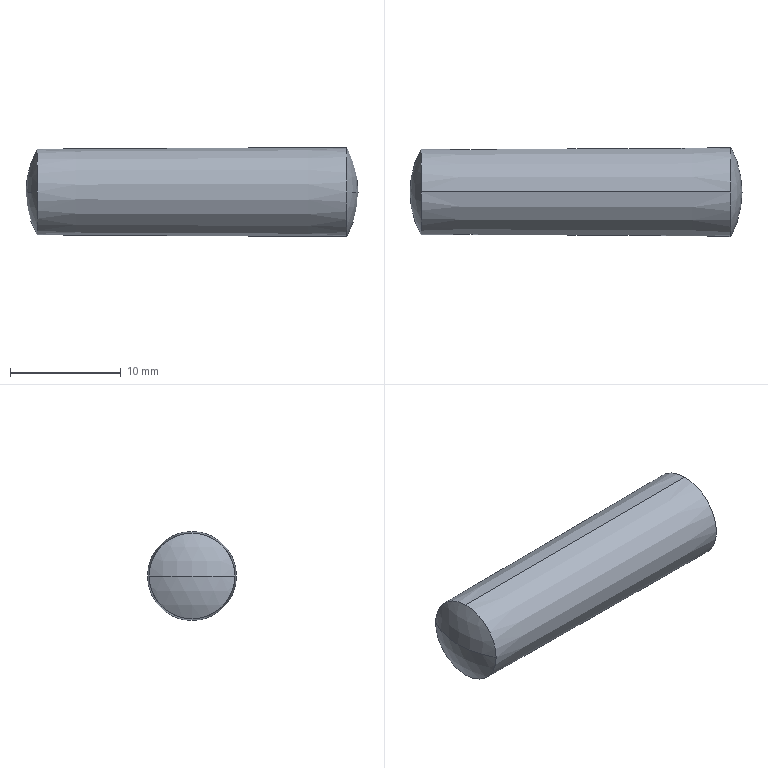Part | SolidWorks | features Revolution 1 | 1 solid | 6 faces | box 30 x 8.048 x 8.048 mm | volume 1422 mm3 | sphere 4 | cone 2
STEP:
#1=CARTESIAN_POINT('',(-7.,0.,3.873));
#2=VERTEX_POINT('',#1);
#3=CARTESIAN_POINT('',(-7.,3.873,0.));
#4=VERTEX_POINT('',#3);
#5=CARTESIAN_POINT('',(-7.,0.,0.));
#6=DIRECTION('',(-1.,0.,0.));
#7=DIRECTION('',(0.,0.,1.));
#8=AXIS2_PLACEMENT_3D('',#5,#6,#7);
#9=CIRCLE('',#8,3.873);
#10=EDGE_CURVE('',#2,#4,#9,.T.);
#11=ORIENTED_EDGE('',*,*,#10,.F.);
#12=CARTESIAN_POINT('',(21.,0.,4.024));
#13=VERTEX_POINT('',#12);
#14=CARTESIAN_POINT('',(21.,0.,4.024));
#15=DIRECTION('',(1.,0.,0.005398));
#16=VECTOR('',#15,1000.);
#17=LINE('',#14,#16);
#18=EDGE_CURVE('',#2,#13,#17,.T.);
#19=ORIENTED_EDGE('',*,*,#18,.T.);
#20=CARTESIAN_POINT('',(21.,4.024,0.));
#21=VERTEX_POINT('',#20);
#22=CARTESIAN_POINT('',(21.,0.,0.));
#23=DIRECTION('',(-1.,0.,0.));
#24=DIRECTION('',(0.,0.,1.));
#25=AXIS2_PLACEMENT_3D('',#22,#23,#24);
#26=CIRCLE('',#25,4.024);
#27=EDGE_CURVE('',#13,#21,#26,.T.);
#28=ORIENTED_EDGE('',*,*,#27,.T.);
#29=CARTESIAN_POINT('',(21.,0.,-4.024));
#30=VERTEX_POINT('',#29);
#31=CARTESIAN_POINT('',(21.,0.,0.));
#32=DIRECTION('',(-1.,0.,0.));
#33=DIRECTION('',(0.,0.,1.));
#34=AXIS2_PLACEMENT_3D('',#31,#32,#33);
#35=CIRCLE('',#34,4.024);
#36=EDGE_CURVE('',#21,#30,#35,.T.);
#37=ORIENTED_EDGE('',*,*,#36,.T.);
#38=CARTESIAN_POINT('',(-7.,0.,-3.873));
#39=VERTEX_POINT('',#38);
#40=CARTESIAN_POINT('',(21.,0.,-4.024));
#41=DIRECTION('',(1.,0.,-0.005398));
#42=VECTOR('',#41,1000.);
#43=LINE('',#40,#42);
#44=EDGE_CURVE('',#39,#30,#43,.T.);
#45=ORIENTED_EDGE('',*,*,#44,.F.);
#46=CARTESIAN_POINT('',(-7.,0.,0.));
#47=DIRECTION('',(-1.,0.,0.));
#48=DIRECTION('',(0.,0.,1.));
#49=AXIS2_PLACEMENT_3D('',#46,#47,#48);
#50=CIRCLE('',#49,3.873);
#51=EDGE_CURVE('',#4,#39,#50,.T.);
#52=ORIENTED_EDGE('',*,*,#51,.F.);
#53=EDGE_LOOP('',(#11,#19,#28,#37,#45,#52));
#54=FACE_OUTER_BOUND('',#53,.T.);
#55=CARTESIAN_POINT('',(21.,0.,0.));
#56=DIRECTION('',(1.,0.,0.));
#57=DIRECTION('',(0.,0.,-1.));
#58=AXIS2_PLACEMENT_3D('',#55,#56,#57);
#59=CONICAL_SURFACE('',#58,4.024,0.005398);
#60=ADVANCED_FACE('',(#54),#59,.T.);
#61=CARTESIAN_POINT('',(22.,0.,0.));
#62=VERTEX_POINT('',#61);
#63=CARTESIAN_POINT('',(13.403,0.,0.));
#64=DIRECTION('',(0.,0.,1.));
#65=DIRECTION('',(1.,0.,0.));
#66=AXIS2_PLACEMENT_3D('',#63,#64,#65);
#67=CIRCLE('',#66,8.597);
#68=EDGE_CURVE('',#62,#21,#67,.T.);
#69=ORIENTED_EDGE('',*,*,#68,.F.);
#70=CARTESIAN_POINT('',(21.,-4.024,0.));
#71=VERTEX_POINT('',#70);
#72=CARTESIAN_POINT('',(13.403,0.,0.));
#73=DIRECTION('',(0.,0.,-1.));
#74=DIRECTION('',(0.,1.,0.));
#75=AXIS2_PLACEMENT_3D('',#72,#73,#74);
#76=CIRCLE('',#75,8.597);
#77=EDGE_CURVE('',#62,#71,#76,.T.);
#78=ORIENTED_EDGE('',*,*,#77,.T.);
#79=CARTESIAN_POINT('',(21.,0.,0.));
#80=DIRECTION('',(-1.,0.,0.));
#81=DIRECTION('',(0.,0.,1.));
#82=AXIS2_PLACEMENT_3D('',#79,#80,#81);
#83=CIRCLE('',#82,4.024);
#84=EDGE_CURVE('',#30,#71,#83,.T.);
#85=ORIENTED_EDGE('',*,*,#84,.F.);
#86=ORIENTED_EDGE('',*,*,#36,.F.);
#87=EDGE_LOOP('',(#69,#78,#85,#86));
#88=FACE_OUTER_BOUND('',#87,.T.);
#89=CARTESIAN_POINT('',(13.403,0.,0.));
#90=DIRECTION('',(0.,0.,-1.));
#91=DIRECTION('',(0.,1.,0.));
#92=AXIS2_PLACEMENT_3D('',#89,#90,#91);
#93=SPHERICAL_SURFACE('',#92,8.597);
#94=ADVANCED_FACE('',(#88),#93,.T.);
#95=ORIENTED_EDGE('',*,*,#51,.T.);
#96=CARTESIAN_POINT('',(-7.,-3.873,0.));
#97=VERTEX_POINT('',#96);
#98=CARTESIAN_POINT('',(-7.,0.,0.));
#99=DIRECTION('',(-1.,0.,0.));
#100=DIRECTION('',(0.,0.,1.));
#101=AXIS2_PLACEMENT_3D('',#98,#99,#100);
#102=CIRCLE('',#101,3.873);
#103=EDGE_CURVE('',#39,#97,#102,.T.);
#104=ORIENTED_EDGE('',*,*,#103,.T.);
#105=CARTESIAN_POINT('',(-8.,0.,0.));
#106=VERTEX_POINT('',#105);
#107=CARTESIAN_POINT('',(0.,0.,0.));
#108=DIRECTION('',(0.,0.,-1.));
#109=DIRECTION('',(0.,1.,0.));
#110=AXIS2_PLACEMENT_3D('',#107,#108,#109);
#111=CIRCLE('',#110,8.);
#112=EDGE_CURVE('',#97,#106,#111,.T.);
#113=ORIENTED_EDGE('',*,*,#112,.T.);
#114=CARTESIAN_POINT('',(0.,0.,0.));
#115=DIRECTION('',(0.,0.,1.));
#116=DIRECTION('',(1.,0.,0.));
#117=AXIS2_PLACEMENT_3D('',#114,#115,#116);
#118=CIRCLE('',#117,8.);
#119=EDGE_CURVE('',#4,#106,#118,.T.);
#120=ORIENTED_EDGE('',*,*,#119,.F.);
#121=EDGE_LOOP('',(#95,#104,#113,#120));
#122=FACE_OUTER_BOUND('',#121,.T.);
#123=CARTESIAN_POINT('',(0.,0.,0.));
#124=DIRECTION('',(0.,0.,-1.));
#125=DIRECTION('',(0.,1.,0.));
#126=AXIS2_PLACEMENT_3D('',#123,#124,#125);
#127=SPHERICAL_SURFACE('',#126,8.);
#128=ADVANCED_FACE('',(#122),#127,.T.);
#129=ORIENTED_EDGE('',*,*,#112,.F.);
#130=CARTESIAN_POINT('',(-7.,0.,0.));
#131=DIRECTION('',(-1.,0.,0.));
#132=DIRECTION('',(0.,0.,1.));
#133=AXIS2_PLACEMENT_3D('',#130,#131,#132);
#134=CIRCLE('',#133,3.873);
#135=EDGE_CURVE('',#97,#2,#134,.T.);
#136=ORIENTED_EDGE('',*,*,#135,.T.);
#137=ORIENTED_EDGE('',*,*,#10,.T.);
#138=ORIENTED_EDGE('',*,*,#119,.T.);
#139=EDGE_LOOP('',(#129,#136,#137,#138));
#140=FACE_OUTER_BOUND('',#139,.T.);
#141=CARTESIAN_POINT('',(0.,0.,0.));
#142=DIRECTION('',(0.,0.,-1.));
#143=DIRECTION('',(0.,1.,0.));
#144=AXIS2_PLACEMENT_3D('',#141,#142,#143);
#145=SPHERICAL_SURFACE('',#144,8.);
#146=ADVANCED_FACE('',(#140),#145,.T.);
#147=ORIENTED_EDGE('',*,*,#77,.F.);
#148=ORIENTED_EDGE('',*,*,#68,.T.);
#149=ORIENTED_EDGE('',*,*,#27,.F.);
#150=CARTESIAN_POINT('',(21.,0.,0.));
#151=DIRECTION('',(-1.,0.,0.));
#152=DIRECTION('',(0.,0.,1.));
#153=AXIS2_PLACEMENT_3D('',#150,#151,#152);
#154=CIRCLE('',#153,4.024);
#155=EDGE_CURVE('',#71,#13,#154,.T.);
#156=ORIENTED_EDGE('',*,*,#155,.F.);
#157=EDGE_LOOP('',(#147,#148,#149,#156));
#158=FACE_OUTER_BOUND('',#157,.T.);
#159=CARTESIAN_POINT('',(13.403,0.,0.));
#160=DIRECTION('',(0.,0.,-1.));
#161=DIRECTION('',(0.,1.,0.));
#162=AXIS2_PLACEMENT_3D('',#159,#160,#161);
#163=SPHERICAL_SURFACE('',#162,8.597);
#164=ADVANCED_FACE('',(#158),#163,.T.);
#165=ORIENTED_EDGE('',*,*,#18,.F.);
#166=ORIENTED_EDGE('',*,*,#135,.F.);
#167=ORIENTED_EDGE('',*,*,#103,.F.);
#168=ORIENTED_EDGE('',*,*,#44,.T.);
#169=ORIENTED_EDGE('',*,*,#84,.T.);
#170=ORIENTED_EDGE('',*,*,#155,.T.);
#171=EDGE_LOOP('',(#165,#166,#167,#168,#169,#170));
#172=FACE_OUTER_BOUND('',#171,.T.);
#173=CARTESIAN_POINT('',(21.,0.,0.));
#174=DIRECTION('',(1.,0.,0.));
#175=DIRECTION('',(0.,0.,-1.));
#176=AXIS2_PLACEMENT_3D('',#173,#174,#175);
#177=CONICAL_SURFACE('',#176,4.024,0.005398);
#178=ADVANCED_FACE('',(#172),#177,.T.);
#179=CLOSED_SHELL('',(#60,#94,#128,#146,#164,#178));
#180=MANIFOLD_SOLID_BREP('',#179);
#181=CARTESIAN_POINT('',(0.,0.,0.));
#182=DIRECTION('',(0.,0.,1.));
#183=DIRECTION('',(1.,0.,0.));
#184=AXIS2_PLACEMENT_3D('',#181,#182,#183);
#185=(LENGTH_UNIT()NAMED_UNIT(*)SI_UNIT(.MILLI.,.METRE.));
#186=UNCERTAINTY_MEASURE_WITH_UNIT(LENGTH_MEASURE(0.00001),#185,'','');
#187=(NAMED_UNIT(*)PLANE_ANGLE_UNIT()SI_UNIT($,.RADIAN.));
#188=(NAMED_UNIT(*)SI_UNIT($,.STERADIAN.)SOLID_ANGLE_UNIT());
#189=(GEOMETRIC_REPRESENTATION_CONTEXT(3)GLOBAL_UNCERTAINTY_ASSIGNED_CONTEXT((#186))GLOBAL_UNIT_ASSIGNED_CONTEXT((#185,#187,#188))REPRESENTATION_CONTEXT('',''));
#190=ADVANCED_BREP_SHAPE_REPRESENTATION('',(#180,#184),#189);